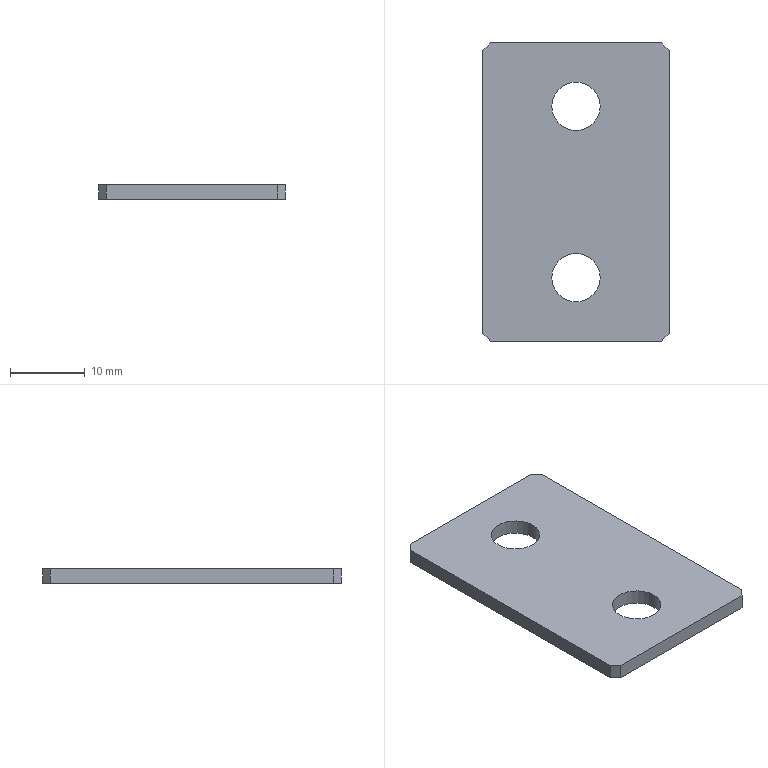Part | NX | 1 solid | 12 faces | box 25 x 40 x 2 mm | volume 1863 mm3 | plane 10 | cylinder 2 | commonest cylinder face diameters 6.5 x2
STEP:
#1=CARTESIAN_POINT('',(3.25,11.5,2.));
#2=VERTEX_POINT('',#1);
#3=CARTESIAN_POINT('',(0.,11.5,2.));
#4=DIRECTION('',(0.,0.,1.));
#5=DIRECTION('',(1.,0.,0.));
#6=AXIS2_PLACEMENT_3D('',#3,#4,#5);
#7=CIRCLE('',#6,3.25);
#8=EDGE_CURVE('',#2,#2,#7,.T.);
#9=ORIENTED_EDGE('',*,*,#8,.F.);
#10=EDGE_LOOP('',(#9));
#11=FACE_BOUND('',#10,.T.);
#12=CARTESIAN_POINT('',(-12.5,19.,2.));
#13=VERTEX_POINT('',#12);
#14=CARTESIAN_POINT('',(-12.5,-19.,2.));
#15=VERTEX_POINT('',#14);
#16=CARTESIAN_POINT('',(-12.5,20.,2.));
#17=DIRECTION('',(0.,-1.,0.));
#18=VECTOR('',#17,1000.);
#19=LINE('',#16,#18);
#20=EDGE_CURVE('',#13,#15,#19,.T.);
#21=ORIENTED_EDGE('',*,*,#20,.T.);
#22=CARTESIAN_POINT('',(-11.5,-20.,2.));
#23=VERTEX_POINT('',#22);
#24=CARTESIAN_POINT('',(-15.75,-15.75,2.));
#25=DIRECTION('',(-0.7071,0.7071,0.));
#26=VECTOR('',#25,1000.);
#27=LINE('',#24,#26);
#28=EDGE_CURVE('',#15,#23,#27,.F.);
#29=ORIENTED_EDGE('',*,*,#28,.T.);
#30=CARTESIAN_POINT('',(11.5,-20.,2.));
#31=VERTEX_POINT('',#30);
#32=CARTESIAN_POINT('',(-12.5,-20.,2.));
#33=DIRECTION('',(1.,0.,0.));
#34=VECTOR('',#33,1000.);
#35=LINE('',#32,#34);
#36=EDGE_CURVE('',#23,#31,#35,.T.);
#37=ORIENTED_EDGE('',*,*,#36,.T.);
#38=CARTESIAN_POINT('',(12.5,-19.,2.));
#39=VERTEX_POINT('',#38);
#40=CARTESIAN_POINT('',(15.75,-15.75,2.));
#41=DIRECTION('',(-0.7071,-0.7071,0.));
#42=VECTOR('',#41,1000.);
#43=LINE('',#40,#42);
#44=EDGE_CURVE('',#31,#39,#43,.F.);
#45=ORIENTED_EDGE('',*,*,#44,.T.);
#46=CARTESIAN_POINT('',(12.5,19.,2.));
#47=VERTEX_POINT('',#46);
#48=CARTESIAN_POINT('',(12.5,20.,2.));
#49=DIRECTION('',(0.,1.,0.));
#50=VECTOR('',#49,1000.);
#51=LINE('',#48,#50);
#52=EDGE_CURVE('',#39,#47,#51,.T.);
#53=ORIENTED_EDGE('',*,*,#52,.T.);
#54=CARTESIAN_POINT('',(11.5,20.,2.));
#55=VERTEX_POINT('',#54);
#56=CARTESIAN_POINT('',(15.75,15.75,2.));
#57=DIRECTION('',(0.7071,-0.7071,0.));
#58=VECTOR('',#57,1000.);
#59=LINE('',#56,#58);
#60=EDGE_CURVE('',#47,#55,#59,.F.);
#61=ORIENTED_EDGE('',*,*,#60,.T.);
#62=CARTESIAN_POINT('',(-11.5,20.,2.));
#63=VERTEX_POINT('',#62);
#64=CARTESIAN_POINT('',(-12.5,20.,2.));
#65=DIRECTION('',(-1.,0.,0.));
#66=VECTOR('',#65,1000.);
#67=LINE('',#64,#66);
#68=EDGE_CURVE('',#55,#63,#67,.T.);
#69=ORIENTED_EDGE('',*,*,#68,.T.);
#70=CARTESIAN_POINT('',(-15.75,15.75,2.));
#71=DIRECTION('',(0.7071,0.7071,0.));
#72=VECTOR('',#71,1000.);
#73=LINE('',#70,#72);
#74=EDGE_CURVE('',#63,#13,#73,.F.);
#75=ORIENTED_EDGE('',*,*,#74,.T.);
#76=EDGE_LOOP('',(#21,#29,#37,#45,#53,#61,#69,#75));
#77=FACE_BOUND('',#76,.T.);
#78=CARTESIAN_POINT('',(3.25,-11.5,2.));
#79=VERTEX_POINT('',#78);
#80=CARTESIAN_POINT('',(0.,-11.5,2.));
#81=DIRECTION('',(0.,0.,1.));
#82=DIRECTION('',(1.,0.,0.));
#83=AXIS2_PLACEMENT_3D('',#80,#81,#82);
#84=CIRCLE('',#83,3.25);
#85=EDGE_CURVE('',#79,#79,#84,.T.);
#86=ORIENTED_EDGE('',*,*,#85,.F.);
#87=EDGE_LOOP('',(#86));
#88=FACE_BOUND('',#87,.T.);
#89=CARTESIAN_POINT('',(0.,0.,2.));
#90=DIRECTION('',(0.,0.,1.));
#91=DIRECTION('',(1.,0.,0.));
#92=AXIS2_PLACEMENT_3D('',#89,#90,#91);
#93=PLANE('',#92);
#94=ADVANCED_FACE('',(#11,#77,#88),#93,.T.);
#95=CARTESIAN_POINT('',(3.25,11.5,0.));
#96=VERTEX_POINT('',#95);
#97=CARTESIAN_POINT('',(0.,11.5,0.));
#98=DIRECTION('',(0.,0.,1.));
#99=DIRECTION('',(1.,0.,0.));
#100=AXIS2_PLACEMENT_3D('',#97,#98,#99);
#101=CIRCLE('',#100,3.25);
#102=EDGE_CURVE('',#96,#96,#101,.T.);
#103=ORIENTED_EDGE('',*,*,#102,.T.);
#104=EDGE_LOOP('',(#103));
#105=FACE_BOUND('',#104,.T.);
#106=CARTESIAN_POINT('',(-11.5,-20.,0.));
#107=VERTEX_POINT('',#106);
#108=CARTESIAN_POINT('',(11.5,-20.,0.));
#109=VERTEX_POINT('',#108);
#110=CARTESIAN_POINT('',(-12.5,-20.,0.));
#111=DIRECTION('',(1.,0.,0.));
#112=VECTOR('',#111,1000.);
#113=LINE('',#110,#112);
#114=EDGE_CURVE('',#107,#109,#113,.T.);
#115=ORIENTED_EDGE('',*,*,#114,.F.);
#116=CARTESIAN_POINT('',(-12.5,-19.,0.));
#117=VERTEX_POINT('',#116);
#118=CARTESIAN_POINT('',(-11.5,-20.,0.));
#119=DIRECTION('',(0.7071,-0.7071,0.));
#120=VECTOR('',#119,1000.);
#121=LINE('',#118,#120);
#122=EDGE_CURVE('',#107,#117,#121,.F.);
#123=ORIENTED_EDGE('',*,*,#122,.T.);
#124=CARTESIAN_POINT('',(-12.5,19.,0.));
#125=VERTEX_POINT('',#124);
#126=CARTESIAN_POINT('',(-12.5,20.,0.));
#127=DIRECTION('',(0.,-1.,0.));
#128=VECTOR('',#127,1000.);
#129=LINE('',#126,#128);
#130=EDGE_CURVE('',#125,#117,#129,.T.);
#131=ORIENTED_EDGE('',*,*,#130,.F.);
#132=CARTESIAN_POINT('',(-11.5,20.,0.));
#133=VERTEX_POINT('',#132);
#134=CARTESIAN_POINT('',(-12.5,19.,0.));
#135=DIRECTION('',(-0.7071,-0.7071,0.));
#136=VECTOR('',#135,1000.);
#137=LINE('',#134,#136);
#138=EDGE_CURVE('',#125,#133,#137,.F.);
#139=ORIENTED_EDGE('',*,*,#138,.T.);
#140=CARTESIAN_POINT('',(11.5,20.,0.));
#141=VERTEX_POINT('',#140);
#142=CARTESIAN_POINT('',(-12.5,20.,0.));
#143=DIRECTION('',(-1.,0.,0.));
#144=VECTOR('',#143,1000.);
#145=LINE('',#142,#144);
#146=EDGE_CURVE('',#141,#133,#145,.T.);
#147=ORIENTED_EDGE('',*,*,#146,.F.);
#148=CARTESIAN_POINT('',(12.5,19.,0.));
#149=VERTEX_POINT('',#148);
#150=CARTESIAN_POINT('',(11.5,20.,0.));
#151=DIRECTION('',(-0.7071,0.7071,0.));
#152=VECTOR('',#151,1000.);
#153=LINE('',#150,#152);
#154=EDGE_CURVE('',#141,#149,#153,.F.);
#155=ORIENTED_EDGE('',*,*,#154,.T.);
#156=CARTESIAN_POINT('',(12.5,-19.,0.));
#157=VERTEX_POINT('',#156);
#158=CARTESIAN_POINT('',(12.5,20.,0.));
#159=DIRECTION('',(0.,1.,0.));
#160=VECTOR('',#159,1000.);
#161=LINE('',#158,#160);
#162=EDGE_CURVE('',#157,#149,#161,.T.);
#163=ORIENTED_EDGE('',*,*,#162,.F.);
#164=CARTESIAN_POINT('',(12.5,-19.,0.));
#165=DIRECTION('',(0.7071,0.7071,0.));
#166=VECTOR('',#165,1000.);
#167=LINE('',#164,#166);
#168=EDGE_CURVE('',#157,#109,#167,.F.);
#169=ORIENTED_EDGE('',*,*,#168,.T.);
#170=EDGE_LOOP('',(#115,#123,#131,#139,#147,#155,#163,#169));
#171=FACE_BOUND('',#170,.T.);
#172=CARTESIAN_POINT('',(3.25,-11.5,0.));
#173=VERTEX_POINT('',#172);
#174=CARTESIAN_POINT('',(0.,-11.5,0.));
#175=DIRECTION('',(0.,0.,1.));
#176=DIRECTION('',(1.,0.,0.));
#177=AXIS2_PLACEMENT_3D('',#174,#175,#176);
#178=CIRCLE('',#177,3.25);
#179=EDGE_CURVE('',#173,#173,#178,.T.);
#180=ORIENTED_EDGE('',*,*,#179,.T.);
#181=EDGE_LOOP('',(#180));
#182=FACE_BOUND('',#181,.T.);
#183=CARTESIAN_POINT('',(0.,0.,0.));
#184=DIRECTION('',(0.,0.,1.));
#185=DIRECTION('',(1.,0.,0.));
#186=AXIS2_PLACEMENT_3D('',#183,#184,#185);
#187=PLANE('',#186);
#188=ADVANCED_FACE('',(#105,#171,#182),#187,.F.);
#189=ORIENTED_EDGE('',*,*,#52,.F.);
#190=CARTESIAN_POINT('',(12.5,-19.,2.));
#191=DIRECTION('',(0.,0.,-1.));
#192=VECTOR('',#191,1000.);
#193=LINE('',#190,#192);
#194=EDGE_CURVE('',#39,#157,#193,.T.);
#195=ORIENTED_EDGE('',*,*,#194,.T.);
#196=ORIENTED_EDGE('',*,*,#162,.T.);
#197=CARTESIAN_POINT('',(12.5,19.,2.));
#198=DIRECTION('',(0.,0.,1.));
#199=VECTOR('',#198,1000.);
#200=LINE('',#197,#199);
#201=EDGE_CURVE('',#149,#47,#200,.T.);
#202=ORIENTED_EDGE('',*,*,#201,.T.);
#203=EDGE_LOOP('',(#189,#195,#196,#202));
#204=FACE_BOUND('',#203,.T.);
#205=CARTESIAN_POINT('',(12.5,20.,2.));
#206=DIRECTION('',(-1.,0.,0.));
#207=DIRECTION('',(0.,-1.,0.));
#208=AXIS2_PLACEMENT_3D('',#205,#206,#207);
#209=PLANE('',#208);
#210=ADVANCED_FACE('',(#204),#209,.F.);
#211=ORIENTED_EDGE('',*,*,#68,.F.);
#212=CARTESIAN_POINT('',(11.5,20.,2.));
#213=DIRECTION('',(0.,0.,-1.));
#214=VECTOR('',#213,1000.);
#215=LINE('',#212,#214);
#216=EDGE_CURVE('',#55,#141,#215,.T.);
#217=ORIENTED_EDGE('',*,*,#216,.T.);
#218=ORIENTED_EDGE('',*,*,#146,.T.);
#219=CARTESIAN_POINT('',(-11.5,20.,2.));
#220=DIRECTION('',(0.,0.,1.));
#221=VECTOR('',#220,1000.);
#222=LINE('',#219,#221);
#223=EDGE_CURVE('',#133,#63,#222,.T.);
#224=ORIENTED_EDGE('',*,*,#223,.T.);
#225=EDGE_LOOP('',(#211,#217,#218,#224));
#226=FACE_BOUND('',#225,.T.);
#227=CARTESIAN_POINT('',(-12.5,20.,2.));
#228=DIRECTION('',(0.,-1.,0.));
#229=DIRECTION('',(0.,0.,-1.));
#230=AXIS2_PLACEMENT_3D('',#227,#228,#229);
#231=PLANE('',#230);
#232=ADVANCED_FACE('',(#226),#231,.F.);
#233=ORIENTED_EDGE('',*,*,#130,.T.);
#234=CARTESIAN_POINT('',(-12.5,-19.,2.));
#235=DIRECTION('',(0.,0.,1.));
#236=VECTOR('',#235,1000.);
#237=LINE('',#234,#236);
#238=EDGE_CURVE('',#117,#15,#237,.T.);
#239=ORIENTED_EDGE('',*,*,#238,.T.);
#240=ORIENTED_EDGE('',*,*,#20,.F.);
#241=CARTESIAN_POINT('',(-12.5,19.,2.));
#242=DIRECTION('',(0.,0.,-1.));
#243=VECTOR('',#242,1000.);
#244=LINE('',#241,#243);
#245=EDGE_CURVE('',#13,#125,#244,.T.);
#246=ORIENTED_EDGE('',*,*,#245,.T.);
#247=EDGE_LOOP('',(#233,#239,#240,#246));
#248=FACE_BOUND('',#247,.T.);
#249=CARTESIAN_POINT('',(-12.5,20.,2.));
#250=DIRECTION('',(1.,0.,0.));
#251=DIRECTION('',(0.,1.,0.));
#252=AXIS2_PLACEMENT_3D('',#249,#250,#251);
#253=PLANE('',#252);
#254=ADVANCED_FACE('',(#248),#253,.F.);
#255=ORIENTED_EDGE('',*,*,#36,.F.);
#256=CARTESIAN_POINT('',(-11.5,-20.,2.));
#257=DIRECTION('',(0.,0.,-1.));
#258=VECTOR('',#257,1000.);
#259=LINE('',#256,#258);
#260=EDGE_CURVE('',#23,#107,#259,.T.);
#261=ORIENTED_EDGE('',*,*,#260,.T.);
#262=ORIENTED_EDGE('',*,*,#114,.T.);
#263=CARTESIAN_POINT('',(11.5,-20.,2.));
#264=DIRECTION('',(0.,0.,1.));
#265=VECTOR('',#264,1000.);
#266=LINE('',#263,#265);
#267=EDGE_CURVE('',#109,#31,#266,.T.);
#268=ORIENTED_EDGE('',*,*,#267,.T.);
#269=EDGE_LOOP('',(#255,#261,#262,#268));
#270=FACE_BOUND('',#269,.T.);
#271=CARTESIAN_POINT('',(-12.5,-20.,2.));
#272=DIRECTION('',(0.,1.,0.));
#273=DIRECTION('',(0.,0.,1.));
#274=AXIS2_PLACEMENT_3D('',#271,#272,#273);
#275=PLANE('',#274);
#276=ADVANCED_FACE('',(#270),#275,.F.);
#277=ORIENTED_EDGE('',*,*,#8,.T.);
#278=EDGE_LOOP('',(#277));
#279=FACE_BOUND('',#278,.T.);
#280=ORIENTED_EDGE('',*,*,#102,.F.);
#281=EDGE_LOOP('',(#280));
#282=FACE_BOUND('',#281,.T.);
#283=CARTESIAN_POINT('',(0.,11.5,2.));
#284=DIRECTION('',(0.,0.,-1.));
#285=DIRECTION('',(-1.,0.,0.));
#286=AXIS2_PLACEMENT_3D('',#283,#284,#285);
#287=CYLINDRICAL_SURFACE('',#286,3.25);
#288=ADVANCED_FACE('',(#279,#282),#287,.F.);
#289=ORIENTED_EDGE('',*,*,#85,.T.);
#290=EDGE_LOOP('',(#289));
#291=FACE_BOUND('',#290,.T.);
#292=ORIENTED_EDGE('',*,*,#179,.F.);
#293=EDGE_LOOP('',(#292));
#294=FACE_BOUND('',#293,.T.);
#295=CARTESIAN_POINT('',(0.,-11.5,2.));
#296=DIRECTION('',(0.,0.,-1.));
#297=DIRECTION('',(-1.,0.,0.));
#298=AXIS2_PLACEMENT_3D('',#295,#296,#297);
#299=CYLINDRICAL_SURFACE('',#298,3.25);
#300=ADVANCED_FACE('',(#291,#294),#299,.F.);
#301=ORIENTED_EDGE('',*,*,#28,.F.);
#302=ORIENTED_EDGE('',*,*,#238,.F.);
#303=ORIENTED_EDGE('',*,*,#122,.F.);
#304=ORIENTED_EDGE('',*,*,#260,.F.);
#305=EDGE_LOOP('',(#301,#302,#303,#304));
#306=FACE_BOUND('',#305,.T.);
#307=CARTESIAN_POINT('',(-11.5,-20.,2.));
#308=DIRECTION('',(0.7071,0.7071,0.));
#309=DIRECTION('',(0.,0.,-1.));
#310=AXIS2_PLACEMENT_3D('',#307,#308,#309);
#311=PLANE('',#310);
#312=ADVANCED_FACE('',(#306),#311,.F.);
#313=ORIENTED_EDGE('',*,*,#44,.F.);
#314=ORIENTED_EDGE('',*,*,#267,.F.);
#315=ORIENTED_EDGE('',*,*,#168,.F.);
#316=ORIENTED_EDGE('',*,*,#194,.F.);
#317=EDGE_LOOP('',(#313,#314,#315,#316));
#318=FACE_BOUND('',#317,.T.);
#319=CARTESIAN_POINT('',(12.5,-19.,2.));
#320=DIRECTION('',(-0.7071,0.7071,0.));
#321=DIRECTION('',(0.,0.,-1.));
#322=AXIS2_PLACEMENT_3D('',#319,#320,#321);
#323=PLANE('',#322);
#324=ADVANCED_FACE('',(#318),#323,.F.);
#325=ORIENTED_EDGE('',*,*,#60,.F.);
#326=ORIENTED_EDGE('',*,*,#201,.F.);
#327=ORIENTED_EDGE('',*,*,#154,.F.);
#328=ORIENTED_EDGE('',*,*,#216,.F.);
#329=EDGE_LOOP('',(#325,#326,#327,#328));
#330=FACE_BOUND('',#329,.T.);
#331=CARTESIAN_POINT('',(11.5,20.,2.));
#332=DIRECTION('',(-0.7071,-0.7071,0.));
#333=DIRECTION('',(0.,0.,-1.));
#334=AXIS2_PLACEMENT_3D('',#331,#332,#333);
#335=PLANE('',#334);
#336=ADVANCED_FACE('',(#330),#335,.F.);
#337=ORIENTED_EDGE('',*,*,#74,.F.);
#338=ORIENTED_EDGE('',*,*,#223,.F.);
#339=ORIENTED_EDGE('',*,*,#138,.F.);
#340=ORIENTED_EDGE('',*,*,#245,.F.);
#341=EDGE_LOOP('',(#337,#338,#339,#340));
#342=FACE_BOUND('',#341,.T.);
#343=CARTESIAN_POINT('',(-12.5,19.,2.));
#344=DIRECTION('',(0.7071,-0.7071,0.));
#345=DIRECTION('',(0.,0.,-1.));
#346=AXIS2_PLACEMENT_3D('',#343,#344,#345);
#347=PLANE('',#346);
#348=ADVANCED_FACE('',(#342),#347,.F.);
#349=CLOSED_SHELL('',(#94,#188,#210,#232,#254,#276,#288,#300,#312,#324,#336,#348));
#350=MANIFOLD_SOLID_BREP('',#349);
#351=(LENGTH_UNIT()NAMED_UNIT(*)SI_UNIT(.MILLI.,.METRE.));
#352=UNCERTAINTY_MEASURE_WITH_UNIT(LENGTH_MEASURE(0.00001),#351,'','');
#353=(NAMED_UNIT(*)PLANE_ANGLE_UNIT()SI_UNIT($,.RADIAN.));
#354=(NAMED_UNIT(*)SI_UNIT($,.STERADIAN.)SOLID_ANGLE_UNIT());
#355=(GEOMETRIC_REPRESENTATION_CONTEXT(3)GLOBAL_UNCERTAINTY_ASSIGNED_CONTEXT((#352))GLOBAL_UNIT_ASSIGNED_CONTEXT((#351,#353,#354))REPRESENTATION_CONTEXT('',''));
#356=ADVANCED_BREP_SHAPE_REPRESENTATION('',(#350),#355);